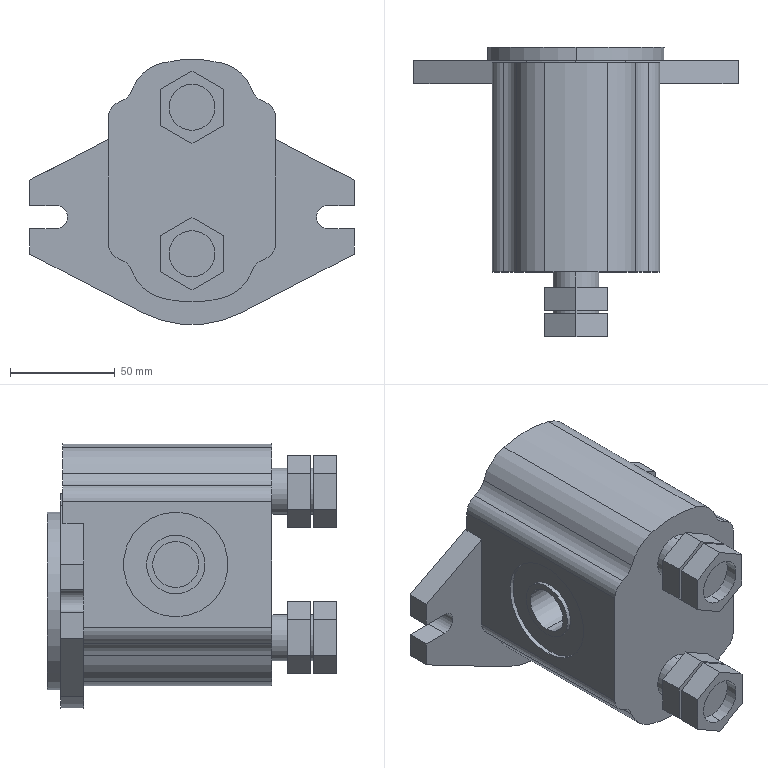Part | SolidWorks | features ICE 9, Extrusion 1, MirrorPattern 1 | 1 solid | 142 faces | box 155 x 138.5 x 127 mm | volume 875484 mm3 | cylinder 72 | plane 70 | commonest cylinder face diameters 22 x16 10 x14 40 x8 20 x6 16 x4 28 x4